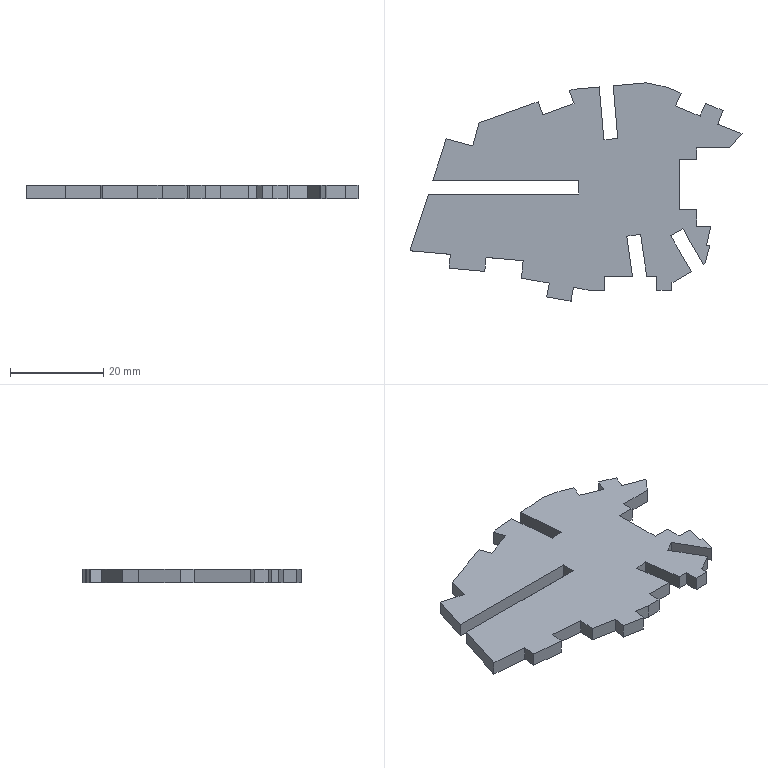Part | SolidWorks | features BaseBody 1 | 1 solid | 65 faces | box 71.254 x 46.863 x 3 mm | volume 5844 mm3 | plane 65